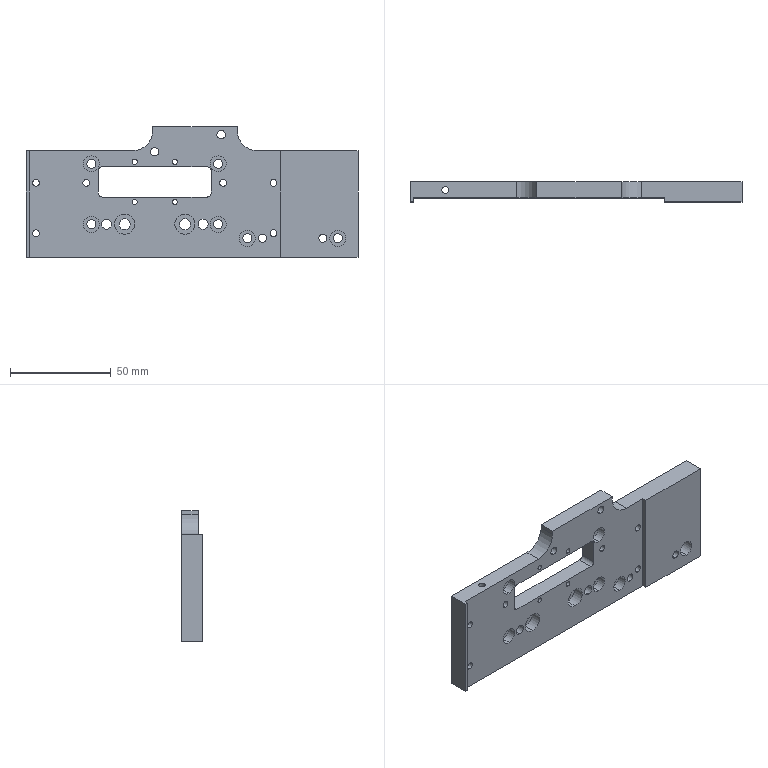Part | STEP file | 11-FG-B01911 | 1 solid | 120 faces | box 165 x 10 x 65 mm | volume 66276 mm3 | cylinder 86 | plane 32 | cone 2 | commonest cylinder face diameters 3.4 x12 4.5 x12 6.5 x12 8 x12 2.5 x8 4 x8